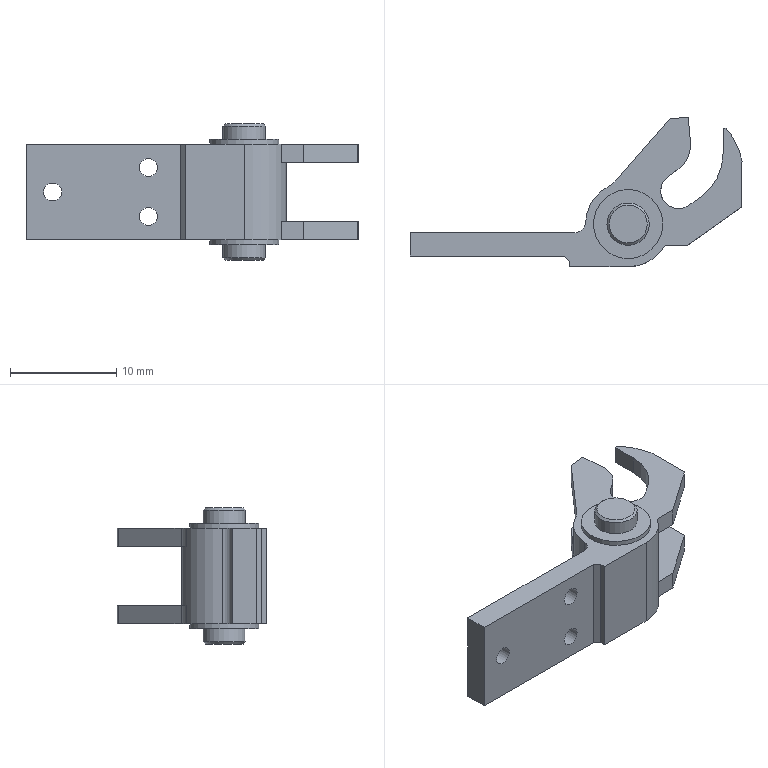NC program | NX | posted with a generic post | part box 31.196 x 14.046 x 12.8 mm
Whole program:
N10 G17 G21 G94 G90
(CAVITY_MILL_1 , TOOL : D5-ROUGH-LOWSPEED)
N12 T00 M6
N14 G54
N16 G17 G0 G90 X34.666 Y-5.142 B0. C0. S15000 M3
N18 G43 Z30. H0
N20 Z11.412
N22 G94 G1 Z9.412 F1000.
N24 X33.299 Y-3.775
N26 G2 X32.714 Y-2.361 R2.
N28 G1 Y-0.781
N30 G3 X31.875 Y0. R3.372
N32 X32.714 Y0.781 R3.372
N34 G1 Y3.869
N36 X32.651
N38 Y2.8
N40 G2 X30.026 Y0.2 R2.622
N42 G1 X29.42
N44 G2 X27.846 Y0.731 R2.6
N46 X26.271 Y0.2 R2.613
N48 G1 X23.322
N50 G2 X20.689 Y2.8 R2.616
N52 G1 Y3.569
N54 X20.623 Y3.567
N56 Y0.783
N58 G3 X21.462 Y0. R3.366
N60 X20.623 Y-0.783 R3.366
N62 G1 Y-3.917
N64 X20.689
N66 Y-2.8
N68 G2 X23.322 Y-0.2 R2.616
N70 G1 X26.271
N72 G2 X27.846 Y-0.731 R2.61
N74 X29.42 Y-0.2 R2.6
N76 G1 X30.026
N78 G2 X32.651 Y-2.8 R2.622
N80 G1 Y-3.94
N82 X32.714
N84 Y-2.361
N86 G2 X33.299 Y-0.947 R2.
N88 G1 X34.714 Y0.468
N90 Z11.412
N92 G0 X34.936 Y-5.116
N94 Z11.024
N96 G1 Z9.024
N98 X33.564 Y-3.745
N100 G2 X32.979 Y-2.331 R2.
N102 G1 X32.875
N104 G2 X32.919 Y-2.791 R2.609
N106 G1 X32.92 Y-2.8
N108 Y-3.941
N110 X32.979
N112 Y-0.769
N114 G3 X32.15 Y0.001 R3.359
N116 X32.979 Y0.772 R3.365
N118 G1 Y3.876
N120 X32.92
N122 Y2.8
N124 G2 X30.305 Y0.2 R2.615
N126 G1 X29.42
N128 G2 X27.863 Y0.718 R2.6
N130 X26.305 Y0.2 R2.608
N132 G1 X22.983
N134 G2 X20.35 Y2.8 R2.616
N136 G1 Y3.56
N138 X20.283 Y3.558
N140 Y0.783
N142 G3 X21.122 Y0. R3.366
N144 X20.283 Y-0.783 R3.366
N146 G1 Y-3.916
N148 X20.35 Y-3.917
N150 Y-2.8
N152 G2 X22.983 Y-0.2 R2.616
N154 G1 X26.305
N156 G2 X27.863 Y-0.718 R2.609
N158 X29.42 Y-0.2 R2.6
N160 G1 X30.301
N162 G2 X32.875 Y-2.331 R2.609
N164 G3 X33.711 Y-3.613 R2.
N166 G1 X34.979 Y-4.482
N168 Z11.024
N170 G0 X35.165 Y-5.077
N172 Z10.636
N174 G1 Z8.636
N176 X33.789 Y-3.7
N178 G2 X33.203 Y-2.286 R2.
N180 G1 X33.094
N182 G2 X33.146 Y-2.8 R2.607
N184 G1 Y-3.943
N186 X33.203
N188 Y-0.764
N190 G3 X32.379 Y0.001 R3.357
N192 X33.203 Y0.767 R3.362
N194 G1 Y3.882
N196 X33.146
N198 Y2.8
N200 G2 X30.538 Y0.2 R2.612
N202 G1 X29.42
N204 G2 X27.88 Y0.705 R2.6
N206 X26.339 Y0.2 R2.603
N208 G1 X22.643
N210 G2 X20.01 Y2.8 R2.616
N212 G1 Y3.551
N214 X19.944 Y3.55
N216 Y0.783
N218 G3 X20.782 Y0. R3.366
N220 X19.944 Y-0.783 R3.366
N222 G1 Y-3.916
N224 X20.01
N226 Y-2.8
N228 G2 X22.643 Y-0.2 R2.616
N230 G1 X26.339
N232 G2 X27.88 Y-0.705 R2.61
N234 X29.42 Y-0.2 R2.6
N236 G1 X30.532
N238 G2 X33.094 Y-2.286 R2.607
N240 G3 X33.951 Y-3.555 R2.
N242 G1 X35.203 Y-4.383
N244 Z10.636
N246 G0 X35.359 Y-5.041
N248 Z10.248
N250 G1 Z8.248
N252 X33.978 Y-3.66
N254 G2 X33.392 Y-2.246 R2.
N256 G1 X33.276
N258 G2 X33.337 Y-2.8 R2.61
N260 G1 Y-3.953
N262 X33.392
N264 Y-0.763
N266 G3 X32.569 Y0. R3.36
N268 X33.392 Y0.765 R3.362
N270 G1 Y3.886
N272 X33.337
N274 Y2.8
N276 G2 X30.733 Y0.2 R2.612
N278 G1 X29.42
N280 G2 X27.888 Y0.7 R2.6
N282 X26.364 Y0.2 R2.528
N284 G1 X22.303
N286 G2 X19.67 Y2.8 R2.617
N288 G1 Y3.543
N290 X19.604 Y3.541
N292 Y0.783
N294 G3 X20.443 Y0. R3.367
N296 X19.604 Y-0.783 R3.367
N298 G1 Y-3.915
N300 X19.67
N302 Y-2.8
N304 G2 X22.303 Y-0.2 R2.617
N306 G1 X26.364
N308 G2 X27.891 Y-0.697 R2.578
N310 X29.42 Y-0.2 R2.6
N312 G1 X30.727
N314 G2 X33.276 Y-2.246 R2.61
N316 G3 X34.153 Y-3.5 R2.
N318 G1 X35.392 Y-4.29
N320 Z10.248
N322 G0 X35.52 Y-5.01
N324 Z9.86
N326 G1 Z7.86
N328 X34.135 Y-3.624
N330 G2 X33.549 Y-2.21 R2.
N332 G1 Y-2.184
N334 X33.548 Y-2.182
N336 X33.427 Y-2.21
N338 G2 X33.496 Y-2.805 R2.606
N340 G1 Y-3.961
N342 X33.549
N344 Y-0.759
N346 G3 X32.73 Y0. R3.356
N348 X33.549 Y0.756 R3.342
N350 G1 Y3.89
N352 X33.496
N354 Y2.799
N356 G2 X31.356 Y0.247 R2.592
N358 X30.893 Y0.2 R3.092
N360 G1 X29.42
N362 G2 X27.888 Y0.7 R2.6
N364 X26.343 Y0.2 R2.503
N366 G1 X21.964
N368 G2 X19.331 Y2.8 R2.619
N370 G1 Y3.534
N372 X19.264 Y3.533
N374 Y0.785
N376 G3 X20.105 Y0. R3.369
N378 X19.264 Y-0.785 R3.369
N380 G1 Y-3.914
N382 X19.331 Y-3.915
N384 Y-2.8
N386 G2 X21.964 Y-0.2 R2.619
N388 G1 X26.343
N390 G2 X27.888 Y-0.699 R2.533
N392 G1 X27.878 Y-0.688
N394 X27.894 Y-0.695
N396 G2 X29.42 Y-0.2 R2.6
N398 G1 X30.889
N400 G2 X33.427 Y-2.21 R2.606
N402 G3 X34.32 Y-3.453 R2.
N404 G1 X35.549 Y-4.215
N406 Z9.86
N408 G0 X35.65 Y-4.983
N410 Z9.472
N412 G1 Z7.472
N414 X34.262 Y-3.595
N416 G2 X33.676 Y-2.18 R2.
N418 G1 X33.668 Y-2.15
N420 X33.547 Y-2.18
N422 G2 X33.624 Y-2.804 R2.61
N424 G1 Y-3.968
N426 X33.676
N428 Y-0.76
N430 G3 X32.854 Y0.001 R3.36
N432 X33.676 Y0.763 R3.365
N434 G1 Y3.894
N436 X33.624
N438 Y2.8
N440 G2 X31.022 Y0.2 R2.615
N442 G1 X29.42
N444 G2 X27.888 Y0.7 R2.6
N446 X26.415 Y0.2 R2.484
N448 G1 X21.624
N450 G2 X18.991 Y2.8 R2.62
N452 G1 Y3.526
N454 X18.925 Y3.524
N456 Y0.785
N458 G3 X19.766 Y0. R3.37
N460 X18.925 Y-0.785 R3.37
N462 G1 Y-3.914
N464 X18.991
N466 Y-2.8
N468 G2 X21.624 Y-0.2 R2.62
N470 G1 X26.448
N472 G2 X27.888 Y-0.699 R2.539
N474 G1 X27.88 Y-0.689
N476 X27.89 Y-0.701
N478 X27.902 Y-0.689
N480 G2 X29.42 Y-0.2 R2.6
N482 G1 X31.02
N484 G2 X33.547 Y-2.18 R2.61
N486 G3 X34.456 Y-3.412 R2.
N488 G1 X35.676 Y-4.146
N490 Z9.472
N492 G0 X35.752 Y-4.961
N494 Z9.084
N496 G1 Z7.084
N498 X34.361 Y-3.57
N500 G2 X33.775 Y-2.156 R2.
N502 G1 X33.764 Y-2.125
N504 X33.643 Y-2.156
N506 G2 X33.724 Y-2.798 R2.601
N508 G1 Y-2.8
N510 Y-3.973
N512 X33.775
N514 Y-0.753
N516 G3 X32.963 Y0. R3.351
N518 X33.775 Y0.753 R3.351
N520 G1 Y3.896
N522 X33.724
N524 Y2.8
N526 G2 X31.122 Y0.2 R2.601
N528 G1 X29.265
N530 G2 X27.89 Y0.686 R2.577
N532 G1 X27.88
N534 X27.84 Y0.658
N536 G2 X26.415 Y0.2 R2.609
N538 G1 X21.284
N540 G2 X18.651 Y2.8 R2.62
N542 G1 Y3.517
N544 X18.585 Y3.516
N546 Y0.785
N548 G3 X19.426 Y0. R3.37
N550 X18.585 Y-0.785 R3.37
N552 G1 Y-3.913
N554 X18.651
N556 Y-2.8
N558 G2 X21.284 Y-0.2 R2.62
N560 G1 X26.448
N562 G2 X27.888 Y-0.699 R2.541
N564 G1 X27.88 Y-0.687
N566 X27.896 Y-0.684
N568 G2 X29.265 Y-0.2 R2.552
N570 G1 X31.122
N572 G2 X33.643 Y-2.156 R2.601
N574 G3 X34.561 Y-3.38 R2.
N576 G1 X35.775 Y-4.1
N578 Z9.084
N580 G0 X35.825 Y-4.945
N582 Z8.696
N584 G1 Z6.696
N586 X34.432 Y-3.552
N588 G2 X33.846 Y-2.138 R2.
N590 G1 X33.831 Y-2.106
N592 X33.71 Y-2.138
N594 G2 X33.796 Y-2.793 R2.6
N596 G1 Y-3.977
N598 X33.846
N600 Y-0.751
N602 G3 X33.035 Y0. R3.35
N604 X33.846 Y0.751 R3.35
N606 G1 Y3.898
N608 X33.796
N610 Y2.8
N612 G2 X31.196 Y0.2 R2.6
N614 G1 X29.265
N616 G2 X27.859 Y0.672 R2.607
N618 X26.415 Y0.2 R2.61
N620 G1 X20.945
N622 G2 X18.312 Y2.8 R2.618
N624 G1 Y3.509
N626 X18.245 Y3.507
N628 Y0.784
N630 G3 X19.085 Y0. R3.368
N632 X18.245 Y-0.784 R3.368
N634 G1 Y-3.912
N636 X18.312 Y-3.913
N638 Y-2.8
N640 Y-2.791
N642 G2 X20.945 Y-0.2 R2.618
N644 G1 X26.448
N646 G2 X27.877 Y-0.684 R2.62
N648 G1 X27.863 Y-0.672
N650 G2 X29.265 Y-0.2 R2.572
N652 G1 X31.196
N654 G2 X33.71 Y-2.138 R2.6
N656 G3 X34.637 Y-3.356 R2.
N658 G1 X35.846 Y-4.062
N660 Z8.696
N662 G0 X35.825 Y-4.945
N664 Z8.308
N666 G1 Z6.308
N668 X34.432 Y-3.552
N670 G2 X33.846 Y-2.138 R2.
N672 G1 X33.831 Y-2.106
N674 X33.71 Y-2.138
N676 G2 X33.796 Y-2.793 R2.6
N678 G1 Y-3.977
N680 X33.846
N682 Y-0.751
N684 G3 X33.035 Y0. R3.35
N686 X33.846 Y0.751 R3.35
N688 G1 Y3.898
N690 X33.796
N692 Y2.8
N694 G2 X31.196 Y0.2 R2.6
N696 G1 X29.265
N698 G2 X27.825 Y0.648 R2.588
N700 X26.415 Y0.2 R2.611
N702 G1 X20.605
N704 G2 X17.972 Y2.8 R2.62
N706 G1 Y3.5
N708 X17.906 Y3.499
N710 Y0.785
N712 G3 X18.747 Y0. R3.37
N714 X17.906 Y-0.785 R3.37
N716 G1 Y-3.912
N718 X17.972
N720 Y-2.8
N722 G2 X20.605 Y-0.2 R2.62
N724 G1 X26.448
N726 G2 X27.827 Y-0.649 R2.619
N728 X29.265 Y-0.2 R2.566
N730 G1 X31.196
N732 G2 X33.71 Y-2.138 R2.6
N734 G3 X34.637 Y-3.356 R2.
N736 G1 X35.846 Y-4.062
N738 Z8.308
N740 G0 X35.825 Y-4.945
N742 Z7.92
N744 G1 Z5.92
N746 X34.432 Y-3.552
N748 G2 X33.846 Y-2.138 R2.
N750 G1 X33.831 Y-2.106
N752 X33.71 Y-2.138
N754 G2 X33.796 Y-2.793 R2.6
N756 G1 Y-3.977
N758 X33.846
N760 Y-0.751
N762 G3 X33.035 Y0. R3.35
N764 X33.846 Y0.751 R3.35
N766 G1 Y3.898
N768 X33.796
N770 Y2.8
N772 G2 X31.196 Y0.2 R2.6
N774 G1 X29.181
N776 G2 X27.772 Y0.613 R2.615
N778 X26.415 Y0.2 R2.605
N780 G1 X20.265
N782 G2 X17.632 Y2.8 R2.623
N784 G1 Y3.492
N786 X17.566 Y3.49
N788 Y0.787
N790 G3 X18.409 Y0. R3.373
N792 X17.566 Y-0.787 R3.373
N794 G1 Y-3.911
N796 X17.632
N798 Y-2.8
N800 G2 X20.265 Y-0.2 R2.623
N802 G1 X26.449
N804 G2 X27.772 Y-0.613 R2.623
N806 X29.181 Y-0.2 R2.627
N808 G1 X31.196
N810 G2 X33.71 Y-2.138 R2.6
N812 G3 X34.637 Y-3.356 R2.
N814 G1 X35.846 Y-4.062
N816 Z7.92
N818 G0 X35.825 Y-4.945
N820 Z7.532
N822 G1 Z5.532
N824 X34.432 Y-3.552
N826 G2 X33.846 Y-2.138 R2.
N828 G1 X33.831 Y-2.106
N830 X33.71 Y-2.138
N832 G2 X33.796 Y-2.793 R2.6
N834 G1 Y-3.977
N836 X33.846
N838 Y-0.751
N840 G3 X33.035 Y0. R3.35
N842 X33.846 Y0.751 R3.35
N844 G1 Y3.898
N846 X33.796
N848 Y2.8
N850 G2 X31.196 Y0.2 R2.6
N852 G1 X29.044
N854 G2 X27.704 Y0.569 R2.623
N856 X26.415 Y0.2 R2.636
N858 G1 X19.926
N860 G2 X17.293 Y2.8 R2.623
N862 G1 Y3.483
N864 X17.226 Y3.481
N866 Y0.787
N868 G3 X18.07 Y0. R3.373
N870 X17.226 Y-0.787 R3.373
N872 G1 Y-3.911
N874 X17.293
N876 Y-2.8
N878 G2 X19.926 Y-0.2 R2.623
N880 G1 X26.449
N882 G2 X27.704 Y-0.569 R2.649
N884 X29.044 Y-0.2 R2.622
N886 G1 X31.196
N888 G2 X33.71 Y-2.138 R2.6
N890 G3 X34.637 Y-3.356 R2.
N892 G1 X35.846 Y-4.062
N894 Z7.532
N896 G0 X35.825 Y-4.945
N898 Z7.144
N900 G1 Z5.144
N902 X34.432 Y-3.552
N904 G2 X33.846 Y-2.138 R2.
N906 G1 X33.831 Y-2.106
N908 X33.71 Y-2.138
N910 G2 X33.796 Y-2.793 R2.6
N912 G1 Y-3.977
N914 X33.846
N916 Y-0.751
N918 G3 X33.035 Y0. R3.35
N920 X33.846 Y0.751 R3.35
N922 G1 Y3.898
N924 X33.796
N926 Y2.8
N928 G2 X31.196 Y0.2 R2.6
N930 G1 X28.871
N932 G2 X27.615 Y0.518 R2.693
N934 X26.415 Y0.2 R2.65
N936 G1 X19.586
N938 G2 X16.953 Y2.8 R2.62
N940 G1 Y3.475
N942 X16.887 Y3.473
N944 Y0.786
N946 G3 X17.728 Y0. R3.37
N948 X16.887 Y-0.786 R3.37
N950 G1 Y-3.91
N952 X16.953
N954 Y-2.8
N956 G2 X19.586 Y-0.2 R2.62
N958 G1 X26.449
N960 G2 X27.617 Y-0.518 R2.666
N962 X28.871 Y-0.2 R2.65
N964 G1 X31.196
N966 G2 X33.71 Y-2.138 R2.6
N968 G3 X34.637 Y-3.356 R2.
N970 G1 X35.846 Y-4.062
N972 Z7.144
N974 G0 X35.825 Y-4.945
N976 Z6.756
N978 G1 Z4.756
N980 X34.432 Y-3.552
N982 G2 X33.846 Y-2.138 R2.
N984 G1 X33.831 Y-2.106
N986 X33.71 Y-2.138
N988 G2 X33.796 Y-2.793 R2.6
N990 G1 Y-3.977
N992 X33.846
N994 Y-0.751
N996 G3 X33.035 Y0. R3.35
N998 X33.846 Y0.751 R3.35
N1000 G1 Y3.898
N1002 X33.796
N1004 Y2.8
N1006 G2 X31.196 Y0.2 R2.6
N1008 G1 X28.644
N1010 G2 X27.501 Y0.461 R2.739
N1012 X26.415 Y0.2 R2.602
N1014 G1 X24.077
N1016 Y-0.2
N1018 X26.449
N1020 G2 X27.508 Y-0.456 R2.863
N1022 G1 X27.633 Y-0.401
N1024 X27.645 Y-0.397
N1026 G2 X28.644 Y-0.2 R2.769
N1028 G1 X31.196
N1030 G2 X33.71 Y-2.138 R2.6
N1032 G3 X34.637 Y-3.356 R2.
N1034 G1 X35.846 Y-4.062
N1036 Z6.756
N1038 G0 X35.825 Y-4.945
N1040 Z6.368
N1042 G1 Z4.368
N1044 X34.432 Y-3.552
N1046 G2 X33.846 Y-2.138 R2.
N1048 G1 X33.831 Y-2.106
N1050 X33.71 Y-2.138
N1052 G2 X33.796 Y-2.793 R2.6
N1054 G1 Y-3.977
N1056 X33.846
N1058 Y-0.751
N1060 G3 X33.035 Y0. R3.35
N1062 X33.846 Y0.751 R3.35
N1064 G1 Y3.898
N1066 X33.796
N1068 Y2.8
N1070 G2 X31.196 Y0.2 R2.6
N1072 G1 X28.371
N1074 G2 X27.366 Y0.398 R2.774
N1076 X26.415 Y0.2 R2.677
N1078 G1 X25.02
N1080 Y-0.2
N1082 X26.449
N1084 G2 X27.363 Y-0.398 R2.671
N1086 X28.371 Y-0.2 R2.924
N1088 G1 X31.196
N1090 G2 X33.71 Y-2.138 R2.6
N1092 G3 X34.637 Y-3.356 R2.
N1094 G1 X35.846 Y-4.062
N1096 Z6.368
N1098 G0 X35.825 Y-4.945
N1100 Z5.98
N1102 G1 Z3.98
N1104 X34.432 Y-3.552
N1106 G2 X33.846 Y-2.138 R2.
N1108 G1 X33.831 Y-2.106
N1110 X33.71 Y-2.138
N1112 G2 X33.796 Y-2.793 R2.6
N1114 G1 Y-3.977
N1116 X33.846
N1118 Y-0.751
N1120 G3 X33.035 Y0. R3.35
N1122 X33.846 Y0.751 R3.35
N1124 G1 Y3.898
N1126 X33.796
N1128 Y2.8
N1130 G2 X31.196 Y0.2 R2.6
N1132 G1 X28.04
N1134 G2 X27.196 Y0.336 R2.946
N1136 X26.415 Y0.2 R2.607
N1138 G1 X25.588
N1140 Y-0.2
N1142 X26.449
N1144 G2 X27.196 Y-0.336 R2.655
N1146 X28.04 Y-0.2 R2.946
N1148 G1 X31.196
N1150 G2 X33.71 Y-2.138 R2.6
N1152 G3 X34.637 Y-3.356 R2.
N1154 G1 X35.846 Y-4.062
N1156 Z5.98
N1158 G0 X35.825 Y-4.945
N1160 Z5.592
N1162 G1 Z3.592
N1164 X34.432 Y-3.552
N1166 G2 X33.846 Y-2.138 R2.
N1168 G1 X33.831 Y-2.106
N1170 X33.71 Y-2.138
N1172 G2 X33.796 Y-2.793 R2.6
N1174 G1 Y-3.977
N1176 X33.846
N1178 Y-0.751
N1180 G3 X33.035 Y0. R3.35
N1182 X33.846 Y0.751 R3.35
N1184 G1 Y3.898
N1186 X33.796
N1188 Y2.8
N1190 G2 X31.196 Y0.2 R2.6
N1192 G1 X27.628
N1194 G2 X26.989 Y0.276 R2.793
N1196 X26.415 Y0.2 R2.531
N1198 G1 X26.002
N1200 Y-0.2
N1202 X26.45
N1204 G2 X26.989 Y-0.276 R2.595
N1206 X27.628 Y-0.2 R2.808
N1208 G1 X31.196
N1210 G2 X33.71 Y-2.138 R2.6
N1212 G3 X34.637 Y-3.356 R2.
N1214 G1 X35.846 Y-4.062
N1216 Z5.592
N1218 G0 X35.825 Y-4.945
N1220 Z5.204
N1222 G1 Z3.204
N1224 X34.432 Y-3.552
N1226 G2 X33.846 Y-2.138 R2.
N1228 G1 X33.831 Y-2.106
N1230 X33.71 Y-2.138
N1232 G2 X33.796 Y-2.793 R2.6
N1234 G1 Y-3.977
N1236 X33.846
N1238 Y-0.751
N1240 G3 X33.035 Y0. R3.35
N1242 X33.846 Y0.751 R3.35
N1244 G1 Y3.898
N1246 X33.796
N1248 Y2.8
N1250 G2 X31.196 Y0.2 R2.6
N1252 G1 X27.121
N1254 X27.059 Y0.201
N1256 X26.737 Y0.226
N1258 G2 X26.321 Y0.196 R3.624
N1260 G1 Y-0.198
N1262 G2 X26.737 Y-0.226 R3.04
N1264 G1 X27.059 Y-0.201
N1266 X27.121 Y-0.2
N1268 X31.196
N1270 G2 X33.71 Y-2.138 R2.6
N1272 G3 X34.637 Y-3.356 R2.
N1274 G1 X35.846 Y-4.062
N1276 Z5.204
N1278 G0 X35.825 Y-4.945
N1280 Z4.816
N1282 G1 Z2.816
N1284 X34.432 Y-3.552
N1286 G2 X33.846 Y-2.138 R2.
N1288 G1 X33.831 Y-2.106
N1290 X33.71 Y-2.138
N1292 G2 X33.796 Y-2.793 R2.6
N1294 G1 Y-3.977
N1296 X33.846
N1298 Y-0.751
N1300 G3 X33.035 Y0. R3.35
N1302 X33.846 Y0.751 R3.35
N1304 G1 Y3.898
N1306 X33.796
N1308 Y2.8
N1310 G2 X31.196 Y0.2 R2.6
N1312 G1 X26.57
N1314 Y-0.2
N1316 X31.196
N1318 G2 X33.71 Y-2.138 R2.6
N1320 G3 X34.637 Y-3.356 R2.
N1322 G1 X35.846 Y-4.062
N1324 Z4.816
N1326 G0 X35.825 Y-4.945
N1328 Z4.428
N1330 G1 Z2.428
N1332 X34.432 Y-3.552
N1334 G2 X33.846 Y-2.138 R2.
N1336 G1 X33.831 Y-2.106
N1338 X33.71 Y-2.138
N1340 G2 X33.796 Y-2.793 R2.6
N1342 G1 Y-3.977
N1344 X33.846
N1346 Y-0.751
N1348 G3 X33.035 Y0. R3.35
N1350 X33.846 Y0.751 R3.35
N1352 G1 Y3.898
N1354 X33.796
N1356 Y2.8
N1358 G2 X31.196 Y0.2 R2.6
N1360 G1 X26.763
N1362 Y-0.2
N1364 X31.196
N1366 G2 X33.71 Y-2.138 R2.6
N1368 G3 X34.637 Y-3.356 R2.
N1370 G1 X35.846 Y-4.062
N1372 Z4.428
N1374 G0 X35.825 Y-4.945
N1376 Z4.04
N1378 G1 Z2.04
N1380 X34.432 Y-3.552
N1382 G2 X33.846 Y-2.138 R2.
N1384 G1 X33.831 Y-2.106
N1386 X33.71 Y-2.138
N1388 G2 X33.796 Y-2.793 R2.6
N1390 G1 Y-3.977
N1392 X33.846
N1394 Y-0.751
N1396 G3 X33.035 Y0. R3.35
N1398 X33.846 Y0.751 R3.35
N1400 G1 Y3.898
N1402 X33.796
N1404 Y2.8
N1406 G2 X31.196 Y0.2 R2.6
N1408 G1 X26.908
N1410 Y-0.2
N1412 X31.196
N1414 G2 X33.71 Y-2.138 R2.6
N1416 G3 X34.637 Y-3.356 R2.
N1418 G1 X35.846 Y-4.062
N1420 Z4.04
N1422 G0 X35.825 Y-4.945
N1424 Z3.652
N1426 G1 Z1.652
N1428 X34.432 Y-3.552
N1430 G2 X33.846 Y-2.138 R2.
N1432 G1 X33.831 Y-2.106
N1434 X33.71 Y-2.138
N1436 G2 X33.796 Y-2.793 R2.6
N1438 G1 Y-3.977
N1440 X33.846
N1442 Y-0.751
N1444 G3 X33.035 Y0. R3.35
N1446 X33.846 Y0.751 R3.35
N1448 G1 Y3.898
N1450 X33.796
N1452 Y2.8
N1454 G2 X31.196 Y0.2 R2.6
N1456 G1 X27.01
N1458 Y-0.2
N1460 X31.196
N1462 G2 X33.71 Y-2.138 R2.6
N1464 G3 X34.637 Y-3.356 R2.
N1466 G1 X35.846 Y-4.062
N1468 Z3.652
N1470 G0 X35.825 Y-4.945
N1472 Z3.264
N1474 G1 Z1.264
N1476 X34.432 Y-3.552
N1478 G2 X33.846 Y-2.138 R2.
N1480 G1 X33.831 Y-2.106
N1482 X33.71 Y-2.138
N1484 G2 X33.796 Y-2.793 R2.6
N1486 G1 Y-3.977
N1488 X33.846
N1490 Y-0.751
N1492 G3 X33.035 Y0. R3.35
N1494 X33.846 Y0.751 R3.35
N1496 G1 Y3.898
N1498 X33.796
N1500 Y2.8
N1502 G2 X31.196 Y0.2 R2.6
N1504 G1 X27.074
N1506 Y-0.2
N1508 X31.196
N1510 G2 X33.71 Y-2.138 R2.6
N1512 G3 X34.637 Y-3.356 R2.
N1514 G1 X35.846 Y-4.062
N1516 Z3.264
N1518 G0 X35.825 Y-4.945
N1520 Z2.876
N1522 G1 Z0.876
N1524 X34.432 Y-3.552
N1526 G2 X33.846 Y-2.138 R2.
N1528 G1 X33.831 Y-2.106
N1530 X33.71 Y-2.138
N1532 G2 X33.796 Y-2.793 R2.6
N1534 G1 Y-3.977
N1536 X33.846
N1538 Y-0.751
N1540 G3 X33.035 Y0. R3.35
N1542 X33.846 Y0.751 R3.35
N1544 G1 Y3.898
N1546 X33.796
N1548 Y2.8
N1550 G2 X31.196 Y0.2 R2.6
N1552 G1 X27.099
N1554 Y0.16
N1556 Y-0.16
N1558 Y-0.2
N1560 X31.196
N1562 G2 X33.71 Y-2.138 R2.6
N1564 G3 X34.637 Y-3.356 R2.
N1566 G1 X35.846 Y-4.062
N1568 Z2.876
N1570 G0 X35.825 Y-4.945
N1572 Z2.488
N1574 G1 Z0.488
N1576 X34.432 Y-3.552
N1578 G2 X33.846 Y-2.138 R2.
N1580 G1 X33.831 Y-2.106
N1582 X33.71 Y-2.138
N1584 G2 X33.796 Y-2.793 R2.6
N1586 G1 Y-3.977
N1588 X33.846
N1590 Y-0.751
N1592 G3 X33.035 Y0. R3.35
N1594 X33.846 Y0.751 R3.35
N1596 G1 Y3.898
N1598 X33.796
N1600 Y2.8
N1602 G2 X31.196 Y0.2 R2.6
N1604 G1 X27.099
N1606 Y-0.2
N1608 X31.196
N1610 G2 X33.71 Y-2.138 R2.6
N1612 G3 X34.637 Y-3.356 R2.
N1614 G1 X35.846 Y-4.062
N1616 Z2.488
N1618 G0 X35.825 Y-4.945
N1620 Z2.1
N1622 G1 Z0.1
N1624 X34.432 Y-3.552
N1626 G2 X33.846 Y-2.138 R2.
N1628 G1 X33.831 Y-2.106
N1630 X33.71 Y-2.138
N1632 G2 X33.796 Y-2.793 R2.6
N1634 G1 Y-3.977
N1636 X33.846
N1638 Y-0.751
N1640 G3 X33.035 Y0. R3.35
N1642 X33.846 Y0.751 R3.35
N1644 G1 Y3.898
N1646 X33.796
N1648 Y2.8
N1650 G2 X31.196 Y0.2 R2.6
N1652 G1 X27.099
N1654 Y-0.2
N1656 X31.196
N1658 G2 X33.71 Y-2.138 R2.6
N1660 G3 X34.637 Y-3.356 R2.
N1662 G1 X35.846 Y-4.062
N1664 Z2.1
N1666 G0 X35.825 Y-4.945
N1668 Z1.733
N1670 G1 Z-0.267
N1672 X34.432 Y-3.552
N1674 G2 X33.846 Y-2.138 R2.
N1676 G1 X33.831 Y-2.106
N1678 X33.71 Y-2.138
N1680 G2 X33.796 Y-2.793 R2.6
N1682 G1 Y-3.977
N1684 X33.846
N1686 Y-0.751
N1688 G3 X33.035 Y0. R3.35
N1690 X33.846 Y0.751 R3.35
N1692 G1 Y3.898
N1694 X33.796
N1696 Y2.8
N1698 G2 X31.196 Y0.2 R2.6
N1700 G1 X27.099
N1702 Y-0.2
N1704 X31.196
N1706 G2 X33.71 Y-2.138 R2.6
N1708 G3 X34.637 Y-3.356 R2.
N1710 G1 X35.846 Y-4.062
N1712 Z1.733
N1714 G0 X35.825 Y-4.945
N1716 Z1.367
N1718 G1 Z-0.633
N1720 X34.432 Y-3.552
N1722 G2 X33.846 Y-2.138 R2.
N1724 G1 X33.831 Y-2.106
N1726 X33.71 Y-2.138
N1728 G2 X33.796 Y-2.793 R2.6
N1730 G1 Y-3.977
N1732 X33.846
N1734 Y-0.751
N1736 G3 X33.035 Y0. R3.35
N1738 X33.846 Y0.751 R3.35
N1740 G1 Y3.898
N1742 X33.796
N1744 Y2.8
N1746 G2 X31.196 Y0.2 R2.6
N1748 G1 X27.099
N1750 Y-0.2
N1752 X31.196
N1754 G2 X33.71 Y-2.138 R2.6
N1756 G3 X34.637 Y-3.356 R2.
N1758 G1 X35.846 Y-4.062
N1760 Z1.367
N1762 G0 X35.825 Y-4.945
N1764 Z1.
N1766 G1 Z-1.
N1768 X34.432 Y-3.552
N1770 G2 X33.846 Y-2.138 R2.
N1772 G1 X33.831 Y-2.106
N1774 X33.71 Y-2.138
N1776 G2 X33.796 Y-2.793 R2.6
N1778 G1 Y-3.977
N1780 X33.846
N1782 Y-0.751
N1784 G3 X33.035 Y0. R3.35
N1786 X33.846 Y0.751 R3.35
N1788 G1 Y3.898
N1790 X33.796
N1792 Y2.8
N1794 G2 X31.196 Y0.2 R2.6
N1796 G1 X27.099
N1798 Y-0.2
N1800 X31.196
N1802 G2 X33.71 Y-2.138 R2.6
N1804 G3 X34.637 Y-3.356 R2.
N1806 G1 X35.846 Y-4.062
N1808 Z1.
N1810 G0 X35.825 Y-4.945
N1812 Z0.633
N1814 G1 Z-1.367
N1816 X34.432 Y-3.552
N1818 G2 X33.846 Y-2.138 R2.
N1820 G1 X33.831 Y-2.106
N1822 X33.71 Y-2.138
N1824 G2 X33.796 Y-2.793 R2.6
N1826 G1 Y-3.977
N1828 X33.846
N1830 Y-0.751
N1832 G3 X33.035 Y0. R3.35
N1834 X33.846 Y0.751 R3.35
N1836 G1 Y3.898
N1838 X33.796
N1840 Y2.8
N1842 G2 X31.196 Y0.2 R2.6
N1844 G1 X27.099
N1846 Y-0.2
N1848 X31.196
N1850 G2 X33.71 Y-2.138 R2.6
N1852 G3 X34.637 Y-3.356 R2.
N1854 G1 X35.846 Y-4.062
N1856 Z0.633
N1858 G0 X35.825 Y-4.945
N1860 Z0.267
N1862 G1 Z-1.733
N1864 X34.432 Y-3.552
N1866 G2 X33.846 Y-2.138 R2.
N1868 G1 X33.831 Y-2.106
N1870 X33.71 Y-2.138
N1872 G2 X33.796 Y-2.793 R2.6
N1874 G1 Y-3.977
N1876 X33.846
N1878 Y-0.751
N1880 G3 X33.035 Y0. R3.35
N1882 X33.846 Y0.751 R3.35
N1884 G1 Y3.898
N1886 X33.796
N1888 Y2.8
N1890 G2 X31.196 Y0.2 R2.6
N1892 G1 X27.099
N1894 Y-0.2
N1896 X31.196
N1898 G2 X33.71 Y-2.138 R2.6
N1900 G3 X34.637 Y-3.356 R2.
N1902 G1 X35.846 Y-4.062
N1904 Z0.267
N1906 G0 X35.825 Y-4.945
N1908 Z-0.1
N1910 G1 Z-2.1
N1912 X34.432 Y-3.552
N1914 G2 X33.846 Y-2.138 R2.
N1916 G1 X33.831 Y-2.106
N1918 X33.71 Y-2.138
N1920 G2 X33.796 Y-2.793 R2.6
N1922 G1 Y-3.977
N1924 X33.846
N1926 Y-0.751
N1928 G3 X33.035 Y0. R3.35
N1930 X33.846 Y0.751 R3.35
N1932 G1 Y3.898
N1934 X33.796
N1936 Y2.8
N1938 G2 X31.196 Y0.2 R2.6
N1940 G1 X27.099
N1942 Y-0.2
N1944 X31.196
N1946 G2 X33.71 Y-2.138 R2.6
N1948 G3 X34.637 Y-3.356 R2.
N1950 G1 X35.846 Y-4.062
N1952 Z-0.1
N1954 G0 X35.825 Y-4.945
N1956 Z-0.467
N1958 G1 Z-2.467
N1960 X34.432 Y-3.552
N1962 G2 X33.846 Y-2.138 R2.
N1964 G1 X33.831 Y-2.106
N1966 X33.71 Y-2.138
N1968 G2 X33.796 Y-2.793 R2.6
N1970 G1 Y-3.977
N1972 X33.846
N1974 Y-0.751
N1976 G3 X33.035 Y0. R3.35
N1978 X33.846 Y0.751 R3.35
N1980 G1 Y3.898
N1982 X33.796
N1984 Y2.8
N1986 G2 X31.196 Y0.2 R2.6
N1988 G1 X27.099
N1990 Y-0.2
N1992 X31.196
N1994 G2 X33.71 Y-2.138 R2.6
N1996 G3 X34.637 Y-3.356 R2.
N1998 G1 X35.846 Y-4.062
N2000 Z-0.467
N2002 G0 X35.825 Y-4.945
N2004 Z-0.833
N2006 G1 Z-2.833
N2008 X34.432 Y-3.552
N2010 G2 X33.846 Y-2.138 R2.
N2012 G1 X33.831 Y-2.106
N2014 X33.71 Y-2.138
N2016 G2 X33.796 Y-2.793 R2.6
N2018 G1 Y-3.977
N2020 X33.846
N2022 Y-0.751
N2024 G3 X33.035 Y0. R3.35
N2026 X33.846 Y0.751 R3.35
N2028 G1 Y3.898
N2030 X33.796
N2032 Y2.8
N2034 G2 X31.196 Y0.2 R2.6
N2036 G1 X27.099
N2038 Y-0.2
N2040 X31.196
N2042 G2 X33.71 Y-2.138 R2.6
N2044 G3 X34.637 Y-3.356 R2.
N2046 G1 X35.846 Y-4.062
N2048 Z-0.833
N2050 G0 X35.825 Y-4.945
N2052 Z-1.2
N2054 G1 Z-3.2
N2056 X34.432 Y-3.552
N2058 G2 X33.846 Y-2.138 R2.
N2060 G1 X33.831 Y-2.106
N2062 X33.71 Y-2.138
N2064 G2 X33.796 Y-2.793 R2.6
N2066 G1 Y-3.977
N2068 X33.846
N2070 Y-0.751
N2072 G3 X33.035 Y0. R3.35
N2074 X33.846 Y0.751 R3.35
N2076 G1 Y3.898
N2078 X33.796
N2080 Y2.8
N2082 G2 X31.196 Y0.2 R2.6
N2084 G1 X27.099
N2086 Y-0.2
N2088 X31.196
N2090 G2 X33.71 Y-2.138 R2.6
N2092 G3 X34.637 Y-3.356 R2.
N2094 G1 X35.846 Y-4.062
N2096 Z-1.2
N2098 G0 Z30.
N2100 X14.518 Y2.606
N2102 Z6.756
N2104 G1 Z4.756
N2106 X15.933 Y1.191
N2108 G2 X16.518 Y-0.223 R2.
N2110 G1 Y-3.909
N2112 X16.595
N2114 Y-2.844
N2116 X16.582 Y-2.833
N2118 G2 X16.923 Y-1.51 R2.564
N2120 G1 Y1.524
N2122 G2 X16.582 Y2.833 R2.448
N2124 G1 X16.595 Y2.845
N2126 Y3.466
N2128 X16.518 Y3.464
N2130 Y-0.223
N2132 G2 X15.933 Y-1.637 R2.
N2134 G1 X14.518 Y-3.051
N2136 Z6.756
N2138 G0 X13.881 Y2.598
N2140 Z6.368
N2142 G1 Z4.368
N2144 X15.295 Y1.184
N2146 G2 X15.881 Y-0.23 R2.
N2148 G1 Y-3.908
N2150 X15.98
N2152 Y3.45
N2154 X15.881 Y3.448
N2156 Y-0.23
N2158 G2 X15.295 Y-1.644 R2.
N2160 G1 X13.881 Y-3.059
N2162 Z6.368
N2164 G0 X13.334 Y2.592
N2166 Z5.98
N2168 G1 Z3.98
N2170 X14.748 Y1.178
N2172 G2 X15.334 Y-0.237 R2.
N2174 G1 Y-3.907
N2176 X15.412
N2178 Y3.436
N2180 X15.334 Y3.434
N2182 Y-0.237
N2184 G2 X14.748 Y-1.651 R2.
N2186 G1 X13.334 Y-3.065
N2188 Z5.98
N2190 G0 X12.93 Y2.592
N2192 Z5.592
N2194 G1 Z3.592
N2196 X14.344 Y1.178
N2198 G2 X14.93 Y-0.237 R2.
N2200 G1 X14.998
N2202 Y3.425
N2204 X14.93 Y3.424
N2206 Y-3.906
N2208 X14.998
N2210 Y-0.237
N2212 G3 X14.412 Y1.178 R2.
N2214 G1 X12.93 Y2.66
N2216 Z5.592
N2218 G0 X12.617 Y2.592
N2220 Z5.204
N2222 G1 Z3.204
N2224 X14.031 Y1.178
N2226 G2 X14.617 Y-0.237 R2.
N2228 G1 X14.679
N2230 Y3.417
N2232 X14.617 Y3.416
N2234 Y-3.905
N2236 X14.679 Y-3.906
N2238 Y-0.237
N2240 G3 X14.093 Y1.178 R2.
N2242 G1 X12.617 Y2.653
N2244 Z5.204
N2246 G0 X12.373 Y2.592
N2248 Z4.816
N2250 G1 Z2.816
N2252 X13.787 Y1.178
N2254 G2 X14.373 Y-0.237 R2.
N2256 G1 X14.43
N2258 Y3.411
N2260 X14.373 Y3.41
N2262 Y-3.905
N2264 X14.43
N2266 Y-0.237
N2268 G3 X13.844 Y1.178 R2.
N2270 G1 X12.373 Y2.649
N2272 Z4.816
N2274 G0 X12.183 Y2.592
N2276 Z4.428
N2278 G1 Z2.428
N2280 X13.597 Y1.178
N2282 G2 X14.183 Y-0.237 R2.
N2284 G1 X14.237
N2286 Y3.406
N2288 X14.183 Y3.405
N2290 Y-3.905
N2292 X14.237
N2294 Y-0.237
N2296 G3 X13.651 Y1.178 R2.
N2298 G1 X12.183 Y2.646
N2300 Z4.428
N2302 G0 X12.04 Y2.592
N2304 Z4.04
N2306 G1 Z2.04
N2308 X13.454 Y1.178
N2310 G2 X14.04 Y-0.237 R2.
N2312 G1 X14.092
N2314 Y3.403
N2316 X14.04 Y3.401
N2318 Y-3.904
N2320 X14.092
N2322 Y-0.237
N2324 G3 X13.506 Y1.178 R2.
N2326 G1 X12.04 Y2.644
N2328 Z4.04
N2330 G0 X11.938 Y2.592
N2332 Z3.652
N2334 G1 Z1.652
N2336 X13.353 Y1.178
N2338 G2 X13.938 Y-0.237 R2.
N2340 G1 X13.99
N2342 Y3.4
N2344 X13.938 Y3.399
N2346 Y-3.904
N2348 X13.99
N2350 Y-0.237
N2352 G3 X13.404 Y1.178 R2.
N2354 G1 X11.938 Y2.643
N2356 Z3.652
N2358 G0 X11.876 Y2.592
N2360 Z3.264
N2362 G1 Z1.264
N2364 X13.29 Y1.178
N2366 G2 X13.876 Y-0.237 R2.
N2368 G1 X13.926
N2370 Y3.398
N2372 X13.876 Y3.397
N2374 Y-3.904
N2376 X13.926
N2378 Y-0.237
N2380 G3 X13.341 Y1.178 R2.
N2382 G1 X11.876 Y2.642
N2384 Z3.264
N2386 G0 X11.845 Y2.592
N2388 Z2.876
N2390 G1 Z0.876
N2392 X13.259 Y1.178
N2394 G2 X13.845 Y-0.237 R2.
N2396 G1 X13.895
N2398 Y3.398
N2400 X13.845 Y3.396
N2402 Y-3.904
N2404 X13.895
N2406 Y-0.237
N2408 G3 X13.31 Y1.178 R2.
N2410 G1 X11.845 Y2.642
N2412 Z2.876
N2414 G0 X11.682 Y2.592
N2416 Z2.488
N2418 G1 Z0.488
N2420 X13.097 Y1.178
N2422 G2 X13.682 Y-0.237 R2.
N2424 G1 X13.744
N2426 Y3.394
N2428 X13.682 Y3.392
N2430 Y-3.904
N2432 X13.744
N2434 Y-0.237
N2436 G3 X13.158 Y1.178 R2.
N2438 G1 X11.682 Y2.654
N2440 Z2.488
N2442 G0 X11.48 Y-9.112
N2444 Z2.1
N2446 G1 Z0.1
N2448 Y-4.485
N2450 G2 X12.895 Y-3.902 R2.
N2452 G1 X13.071 Y-3.903
N2454 Y3.377
N2456 X12.759 Y3.369
N2458 X12.719 Y-3.902
N2460 X12.895
N2462 G2 X12.971 Y-3.519 R1.
N2464 G1 Y-9.112
N2466 Z2.1
N2468 G0 Z30.
N2470 M5
N2472 M2